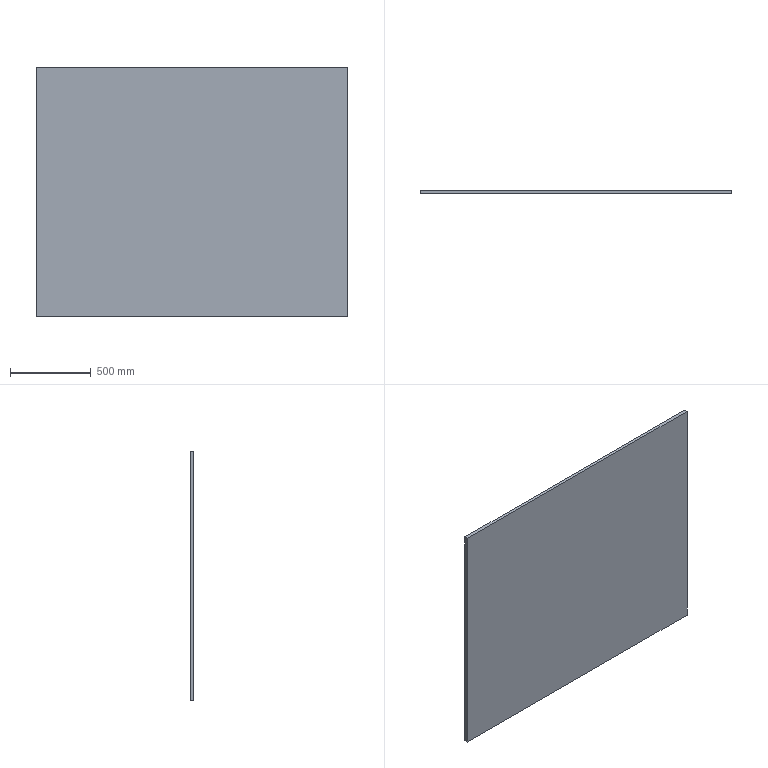Part | STEP file | 果蔬烘干机框架-106 | 1 solid | 6 faces | box 1920 x 20 x 1540 mm | volume 59136000 mm3 | plane 6
STEP:
#1=CARTESIAN_POINT('',(960.,0.,770.));
#2=VERTEX_POINT('',#1);
#3=CARTESIAN_POINT('',(960.,0.,-770.));
#4=VERTEX_POINT('',#3);
#5=CARTESIAN_POINT('',(960.,0.,-770.));
#6=DIRECTION('',(0.,0.,-1.));
#7=VECTOR('',#6,1000.);
#8=LINE('',#5,#7);
#9=EDGE_CURVE('',#2,#4,#8,.T.);
#10=ORIENTED_EDGE('',*,*,#9,.T.);
#11=CARTESIAN_POINT('',(960.,20.,-770.));
#12=VERTEX_POINT('',#11);
#13=CARTESIAN_POINT('',(960.,20.,-770.));
#14=DIRECTION('',(0.,-1.,0.));
#15=VECTOR('',#14,1000.);
#16=LINE('',#13,#15);
#17=EDGE_CURVE('',#12,#4,#16,.T.);
#18=ORIENTED_EDGE('',*,*,#17,.F.);
#19=CARTESIAN_POINT('',(960.,20.,770.));
#20=VERTEX_POINT('',#19);
#21=CARTESIAN_POINT('',(960.,20.,-770.));
#22=DIRECTION('',(0.,0.,-1.));
#23=VECTOR('',#22,1000.);
#24=LINE('',#21,#23);
#25=EDGE_CURVE('',#20,#12,#24,.T.);
#26=ORIENTED_EDGE('',*,*,#25,.F.);
#27=CARTESIAN_POINT('',(960.,20.,770.));
#28=DIRECTION('',(0.,-1.,0.));
#29=VECTOR('',#28,1000.);
#30=LINE('',#27,#29);
#31=EDGE_CURVE('',#20,#2,#30,.T.);
#32=ORIENTED_EDGE('',*,*,#31,.T.);
#33=EDGE_LOOP('',(#10,#18,#26,#32));
#34=FACE_OUTER_BOUND('',#33,.T.);
#35=CARTESIAN_POINT('',(960.,20.,-770.));
#36=DIRECTION('',(-1.,0.,0.));
#37=DIRECTION('',(0.,0.,1.));
#38=AXIS2_PLACEMENT_3D('',#35,#36,#37);
#39=PLANE('',#38);
#40=ADVANCED_FACE('',(#34),#39,.F.);
#41=CARTESIAN_POINT('',(-960.,0.,-770.));
#42=VERTEX_POINT('',#41);
#43=CARTESIAN_POINT('',(-960.,0.,-770.));
#44=DIRECTION('',(-1.,0.,0.));
#45=VECTOR('',#44,1000.);
#46=LINE('',#43,#45);
#47=EDGE_CURVE('',#4,#42,#46,.T.);
#48=ORIENTED_EDGE('',*,*,#47,.T.);
#49=CARTESIAN_POINT('',(-960.,20.,-770.));
#50=VERTEX_POINT('',#49);
#51=CARTESIAN_POINT('',(-960.,20.,-770.));
#52=DIRECTION('',(0.,-1.,0.));
#53=VECTOR('',#52,1000.);
#54=LINE('',#51,#53);
#55=EDGE_CURVE('',#50,#42,#54,.T.);
#56=ORIENTED_EDGE('',*,*,#55,.F.);
#57=CARTESIAN_POINT('',(-960.,20.,-770.));
#58=DIRECTION('',(-1.,0.,0.));
#59=VECTOR('',#58,1000.);
#60=LINE('',#57,#59);
#61=EDGE_CURVE('',#12,#50,#60,.T.);
#62=ORIENTED_EDGE('',*,*,#61,.F.);
#63=ORIENTED_EDGE('',*,*,#17,.T.);
#64=EDGE_LOOP('',(#48,#56,#62,#63));
#65=FACE_OUTER_BOUND('',#64,.T.);
#66=CARTESIAN_POINT('',(-960.,20.,-770.));
#67=DIRECTION('',(0.,0.,1.));
#68=DIRECTION('',(1.,0.,0.));
#69=AXIS2_PLACEMENT_3D('',#66,#67,#68);
#70=PLANE('',#69);
#71=ADVANCED_FACE('',(#65),#70,.F.);
#72=CARTESIAN_POINT('',(-960.,0.,770.));
#73=VERTEX_POINT('',#72);
#74=CARTESIAN_POINT('',(-960.,0.,-770.));
#75=DIRECTION('',(0.,0.,1.));
#76=VECTOR('',#75,1000.);
#77=LINE('',#74,#76);
#78=EDGE_CURVE('',#42,#73,#77,.T.);
#79=ORIENTED_EDGE('',*,*,#78,.T.);
#80=CARTESIAN_POINT('',(-960.,20.,770.));
#81=VERTEX_POINT('',#80);
#82=CARTESIAN_POINT('',(-960.,20.,770.));
#83=DIRECTION('',(0.,-1.,0.));
#84=VECTOR('',#83,1000.);
#85=LINE('',#82,#84);
#86=EDGE_CURVE('',#81,#73,#85,.T.);
#87=ORIENTED_EDGE('',*,*,#86,.F.);
#88=CARTESIAN_POINT('',(-960.,20.,-770.));
#89=DIRECTION('',(0.,0.,1.));
#90=VECTOR('',#89,1000.);
#91=LINE('',#88,#90);
#92=EDGE_CURVE('',#50,#81,#91,.T.);
#93=ORIENTED_EDGE('',*,*,#92,.F.);
#94=ORIENTED_EDGE('',*,*,#55,.T.);
#95=EDGE_LOOP('',(#79,#87,#93,#94));
#96=FACE_OUTER_BOUND('',#95,.T.);
#97=CARTESIAN_POINT('',(-960.,20.,-770.));
#98=DIRECTION('',(1.,0.,0.));
#99=DIRECTION('',(0.,0.,-1.));
#100=AXIS2_PLACEMENT_3D('',#97,#98,#99);
#101=PLANE('',#100);
#102=ADVANCED_FACE('',(#96),#101,.F.);
#103=CARTESIAN_POINT('',(-960.,0.,770.));
#104=DIRECTION('',(1.,0.,0.));
#105=VECTOR('',#104,1000.);
#106=LINE('',#103,#105);
#107=EDGE_CURVE('',#73,#2,#106,.T.);
#108=ORIENTED_EDGE('',*,*,#107,.T.);
#109=ORIENTED_EDGE('',*,*,#31,.F.);
#110=CARTESIAN_POINT('',(-960.,20.,770.));
#111=DIRECTION('',(1.,0.,0.));
#112=VECTOR('',#111,1000.);
#113=LINE('',#110,#112);
#114=EDGE_CURVE('',#81,#20,#113,.T.);
#115=ORIENTED_EDGE('',*,*,#114,.F.);
#116=ORIENTED_EDGE('',*,*,#86,.T.);
#117=EDGE_LOOP('',(#108,#109,#115,#116));
#118=FACE_OUTER_BOUND('',#117,.T.);
#119=CARTESIAN_POINT('',(-960.,20.,770.));
#120=DIRECTION('',(0.,0.,-1.));
#121=DIRECTION('',(-1.,0.,0.));
#122=AXIS2_PLACEMENT_3D('',#119,#120,#121);
#123=PLANE('',#122);
#124=ADVANCED_FACE('',(#118),#123,.F.);
#125=ORIENTED_EDGE('',*,*,#25,.T.);
#126=ORIENTED_EDGE('',*,*,#61,.T.);
#127=ORIENTED_EDGE('',*,*,#92,.T.);
#128=ORIENTED_EDGE('',*,*,#114,.T.);
#129=EDGE_LOOP('',(#125,#126,#127,#128));
#130=FACE_OUTER_BOUND('',#129,.T.);
#131=CARTESIAN_POINT('',(0.,20.,0.));
#132=DIRECTION('',(0.,1.,0.));
#133=DIRECTION('',(0.,0.,1.));
#134=AXIS2_PLACEMENT_3D('',#131,#132,#133);
#135=PLANE('',#134);
#136=ADVANCED_FACE('',(#130),#135,.T.);
#137=ORIENTED_EDGE('',*,*,#9,.F.);
#138=ORIENTED_EDGE('',*,*,#107,.F.);
#139=ORIENTED_EDGE('',*,*,#78,.F.);
#140=ORIENTED_EDGE('',*,*,#47,.F.);
#141=EDGE_LOOP('',(#137,#138,#139,#140));
#142=FACE_OUTER_BOUND('',#141,.T.);
#143=CARTESIAN_POINT('',(0.,0.,0.));
#144=DIRECTION('',(0.,1.,0.));
#145=DIRECTION('',(0.,0.,1.));
#146=AXIS2_PLACEMENT_3D('',#143,#144,#145);
#147=PLANE('',#146);
#148=ADVANCED_FACE('',(#142),#147,.F.);
#149=CLOSED_SHELL('',(#40,#71,#102,#124,#136,#148));
#150=MANIFOLD_SOLID_BREP('',#149);
#151=CARTESIAN_POINT('',(0.,0.,0.));
#152=DIRECTION('',(0.,0.,1.));
#153=DIRECTION('',(1.,0.,0.));
#154=AXIS2_PLACEMENT_3D('',#151,#152,#153);
#155=(LENGTH_UNIT()NAMED_UNIT(*)SI_UNIT(.MILLI.,.METRE.));
#156=UNCERTAINTY_MEASURE_WITH_UNIT(LENGTH_MEASURE(0.00001),#155,'','');
#157=(NAMED_UNIT(*)PLANE_ANGLE_UNIT()SI_UNIT($,.RADIAN.));
#158=(NAMED_UNIT(*)SI_UNIT($,.STERADIAN.)SOLID_ANGLE_UNIT());
#159=(GEOMETRIC_REPRESENTATION_CONTEXT(3)GLOBAL_UNCERTAINTY_ASSIGNED_CONTEXT((#156))GLOBAL_UNIT_ASSIGNED_CONTEXT((#155,#157,#158))REPRESENTATION_CONTEXT('',''));
#160=ADVANCED_BREP_SHAPE_REPRESENTATION('',(#150,#154),#159);